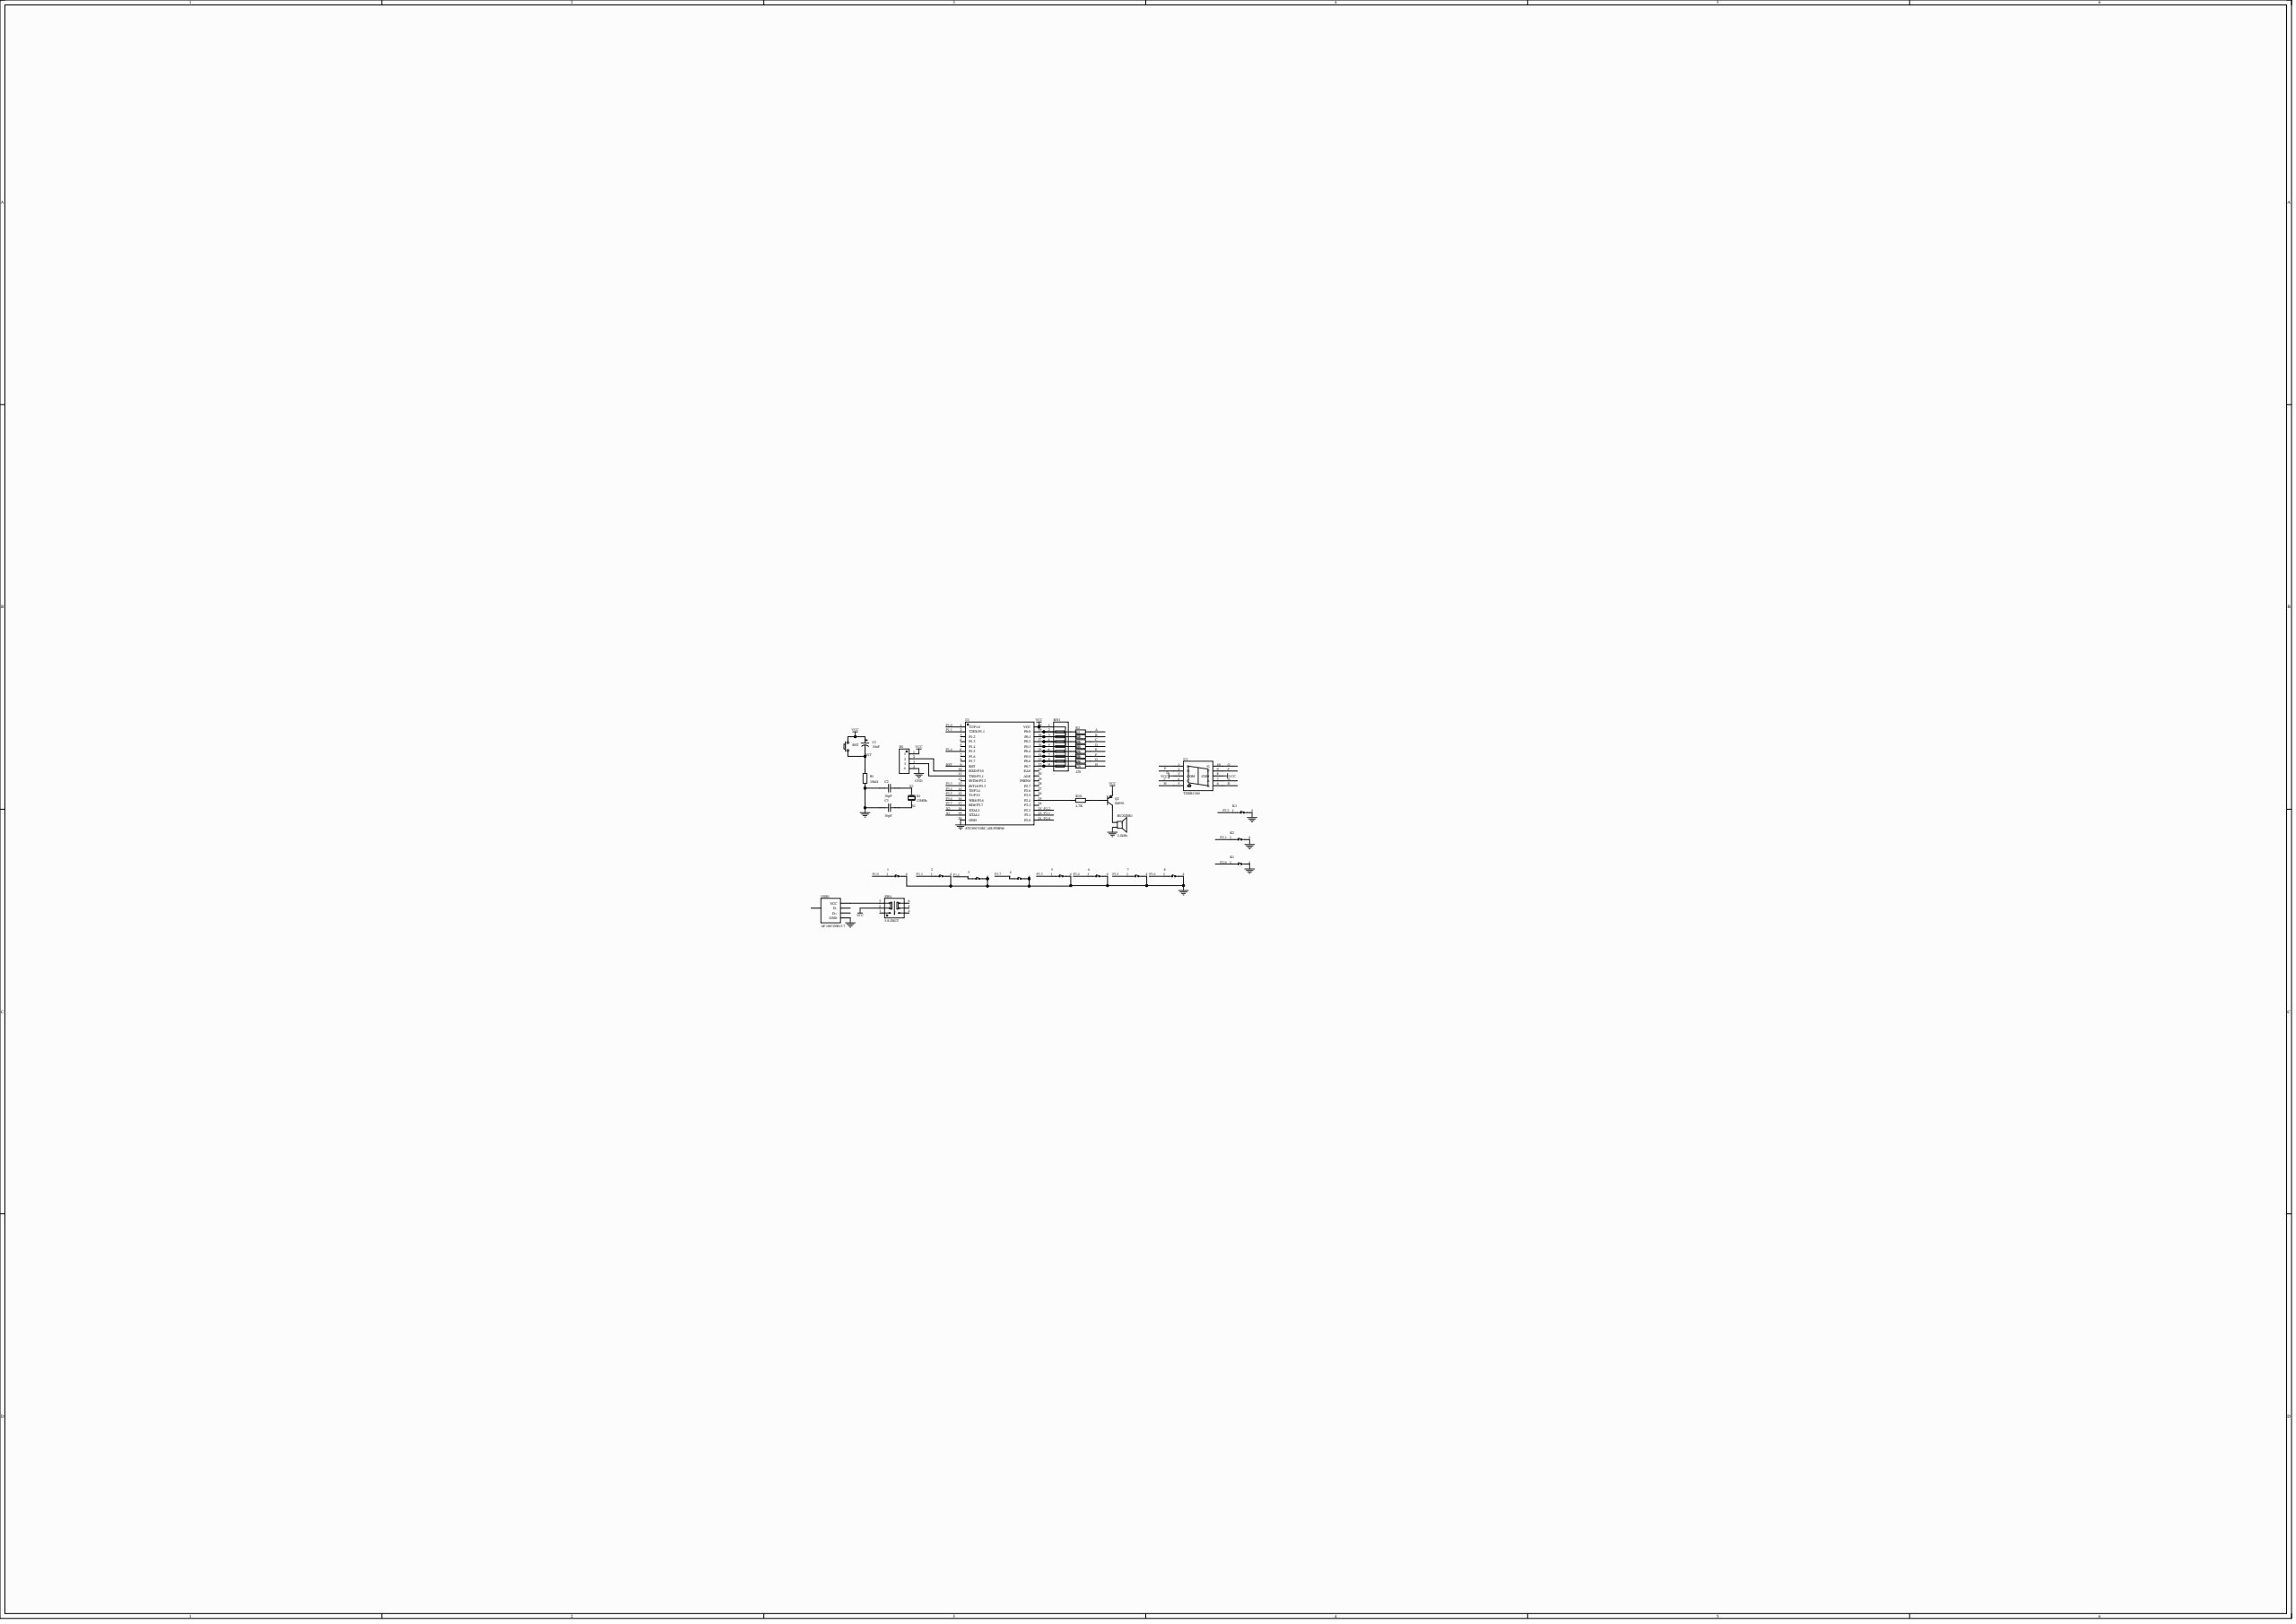Circuit board | Altium Designer | 34 parts | 38 nets
Bill of materials:
Comment,Description,Designator,Footprint,LibRef,Quantity
"TS665CJ","Circuit structure: SPST; button shape: round button; actuating force: 2.5N; mounting: through-hole; switch length: 6mm; switch width: 6mm; switch height: 5mm; with bracket: no bracket; contact current: 50mA; rated voltage: 12V; with lamp: none; operating life: 5 ten-thousand cycles;","1, 2, 3, 4, 5, 6, 7, 8, K1, K2, K3","SW-TH_4P-L6.0-W6.0-P4.50-LS6.5","TS665CJ","11"
"2.4kHz","Drive mode: active (built-in driver circuit); construction type: electromagnetic; rated voltage: 5V; frequency: 2.4kHz; sound pressure level (SPL): 85dB;","BUZZER1","BUZ-TH_BD12.0-P7.60-D0.6-FD","TMB12A05_C96093","1"
"10uF","Capacitance: 10uF; tolerance: ±20%; rated voltage: 400V; ripple current: 160mA@100kHz; equivalent series resistance (ESR): -;","C1","CAP-TH_BD8.0-P3.50-D0.6-FD","ERK2GM100F12OT","1"
"30pF","Capacitance: 30pF; tolerance: ±5%; rated voltage: 50V; temperature coefficient: C0G;","C2, C3","CAP-TH_L8.5-W5.0-P5.00-D1.2","CC4-0805N300J500F3","2"
"","","H1","HDR-TH_4P-P2.54-V-F","HDR-F_2.54_1x4P","1"
"S8550","Transistor type: PNP; collector current (Ic): 500mA; collector-emitter breakdown voltage (Vceo): 25V; power dissipation (Pd): 625mW; DC current gain (hFE): 160@50mA,1V;","Q2","TO-92-3_L4.5-W3.5-P1.27-L","S8550_C2931493","1"
"10kΩ","Resistor type: metal film resistor; resistance: 10kΩ; tolerance: ±1%; power: 250mW; temperature coefficient: ±50ppm/?;","R1","RES-TH_BD2.4-L6.3-P10.30-D0.6","MFR-25FTE52-10K","1"
"470","","R2, R3, R4, R5, R6, R7, R8, R9","R0603","Res_0603","8"
"4.7K","Resistor type: metal film resistor; resistance: 470Ω; tolerance: ±1%; power: 250mW; temperature coefficient: ±50ppm/?;","R10","RES-TH_BD2.2-L6.5-P10.50-D0.6","MFR0W4F4700A50","1"
"-","Number of resistors: -; resistance: -; power per element: -;","RN1","RES-ARRAY-TH_9P-P2.54-D1.0","排阻 10 K 5%","1"
"","","RST","Key_TH_3.5x6x4.3","Key_TH_3.5x6x4.3","1"
"5.8 ZSGT","Circuit structure: DPDT; self-lock/no-lock: self-lock; mounting: through-hole; contact current: 110mA; rated voltage: 30V; with lamp: no; actuating force: 1.5N; operating life: 10 ten-thousand cycles;","SW4","SW-TH_5.8ZSGT","5.8 ZSGT","1"
"STC89C52RC-40I-PDIP40","CPU core: 51 family; CPU max frequency: -;","U1","DIP-40_L52.0-W13.7-P2.54-LS15.2-BL","STC89C52RC-40I-PDIP40","1"
"TDSR1360","Digits: 1; power dissipation (Pd): 185mW; emitting color: red; LED polarity: common cathode; digit/letter size (inch): 0.51;","U2","LED-SEG-TH_10P-L17.6-W12.4-P2.54-S15.24-BL","TDSR1360","1"
"AF 180°ZJB13.7","","USB1","USB-A-TH_AF-ZJB13.7","AF 180°ZJB13.7","1"
"12MHz","Crystal type: through-hole crystal; frequency: 12MHz; normal temperature frequency deviation: ±20ppm; load capacitance: 20pF; frequency stability: ±30ppm;","X1","HC-49US_L11.5-W4.5-P4.88","X49SD12MSD2SC","1"
Netlist (Protel format):
[
1
SW-TH_4P-L6.0-W6.0-P4.50-LS6.5
TS665CJ



]
[
2
SW-TH_4P-L6.0-W6.0-P4.50-LS6.5
TS665CJ



]
[
3
SW-TH_4P-L6.0-W6.0-P4.50-LS6.5
TS665CJ



]
[
4
SW-TH_4P-L6.0-W6.0-P4.50-LS6.5
TS665CJ



]
[
5
SW-TH_4P-L6.0-W6.0-P4.50-LS6.5
TS665CJ



]
[
6
SW-TH_4P-L6.0-W6.0-P4.50-LS6.5
TS665CJ



]
[
7
SW-TH_4P-L6.0-W6.0-P4.50-LS6.5
TS665CJ



]
[
8
SW-TH_4P-L6.0-W6.0-P4.50-LS6.5
TS665CJ



]
[
BUZZER1
BUZ-TH_BD12.0-P7.60-D0.6-FD
2.4kHz



]
[
C1
CAP-TH_BD8.0-P3.50-D0.6-FD
10uF



]
[
C2
CAP-TH_L8.5-W5.0-P5.00-D1.2
30pF



]
[
C3
CAP-TH_L8.5-W5.0-P5.00-D1.2
30pF



]
[
H1
HDR-TH_4P-P2.54-V-F




]
[
K1
SW-TH_4P-L6.0-W6.0-P4.50-LS6.5
TS665CJ



]
[
K2
SW-TH_4P-L6.0-W6.0-P4.50-LS6.5
TS665CJ



]
[
K3
SW-TH_4P-L6.0-W6.0-P4.50-LS6.5
TS665CJ



]
[
Q2
TO-92-3_L4.5-W3.5-P1.27-L
S8550



]
[
R1
RES-TH_BD2.4-L6.3-P10.30-D0.6
10kΩ



]
[
R2
R0603
470



]
[
R3
R0603
470



]
[
R4
R0603
470



]
[
R5
R0603
470



]
[
R6
R0603
470



]
[
R7
R0603
470



]
[
R8
R0603
470



]
[
R9
R0603
470



]
[
R10
RES-TH_BD2.2-L6.5-P10.50-D0.6
4.7K



]
[
RN1
RES-ARRAY-TH_9P-P2.54-D1.0
-



]
[
RST
Key_TH_3.5x6x4.3




]
[
SW4
SW-TH_5.8ZSGT
5.8 ZSGT



]
[
U1
DIP-40_L52.0-W13.7-P2.54-LS15.2-BL
STC89C52RC-40I-PDIP40



]
[
U2
LED-SEG-TH_10P-L17.6-W12.4-P2.54-S15.24-BL
TDSR1360



]
[
USB1
USB-A-TH_AF-ZJB13.7
AF 180°ZJB13.7



]
[
X1
HC-49US_L11.5-W4.5-P4.88
12MHz



]
(
X2
C2-2
U1-18
X1-1
)
(
X1
C3-2
U1-19
X1-2
)
(
VCC
C1-1
H1-1
Q2-1
RN1-1
RST-B
SW4-2
U1-40
U2-3
U2-8
)
(
RST
C1-2
R1-2
RST-A
U1-9
)
(
P3.7
4-1
U1-17
)
(
P3.6
8-1
U1-16
)
(
P3.5
7-1
U1-15
)
(
P3.4
6-1
U1-14
)
(
P3.3
5-1
U1-13
)
(
P2.2
K3-1
U1-23
)
(
P2.1
K2-1
U1-22
)
(
P2.0
K1-1
U1-21
)
(
P1.4
3-1
U1-6
)
(
P1.1
2-1
U1-2
)
(
P1.0
1-1
U1-1
)
(
NetSW4_3
SW4-3
USB1-1
)
(
NetR10_1
R10-1
U1-25
)
(
NetR9_1
R9-1
RN1-9
U1-32
)
(
NetR8_1
R8-1
RN1-8
U1-33
)
(
NetR7_1
R7-1
RN1-7
U1-34
)
(
NetR6_1
R6-1
RN1-6
U1-35
)
(
NetR5_1
R5-1
RN1-5
U1-36
)
(
NetR4_1
R4-1
RN1-4
U1-37
)
(
NetR3_1
R3-1
RN1-3
U1-38
)
(
NetR2_1
R2-1
RN1-2
U1-39
)
(
NetQ2_2
Q2-2
R10-2
)
(
NetH1_3
H1-3
U1-11
)
(
NetH1_2
H1-2
U1-10
)
(
NetBUZZER1_1
BUZZER1-1
Q2-3
)
(
H
R9-2
U2-5
)
(
GND
1-4
2-4
3-4
4-4
5-4
6-4
7-4
8-4
BUZZER1-2
C2-1
C3-1
H1-4
K1-4
K2-4
K3-4
R1-1
U1-20
USB1-4
)
(
G
R8-2
U2-10
)
(
F
R7-2
U2-9
)
(
E
R6-2
U2-1
)
(
D
R5-2
U2-2
)
(
C
R4-2
U2-4
)
(
B
R3-2
U2-6
)
(
A
R2-2
U2-7
)